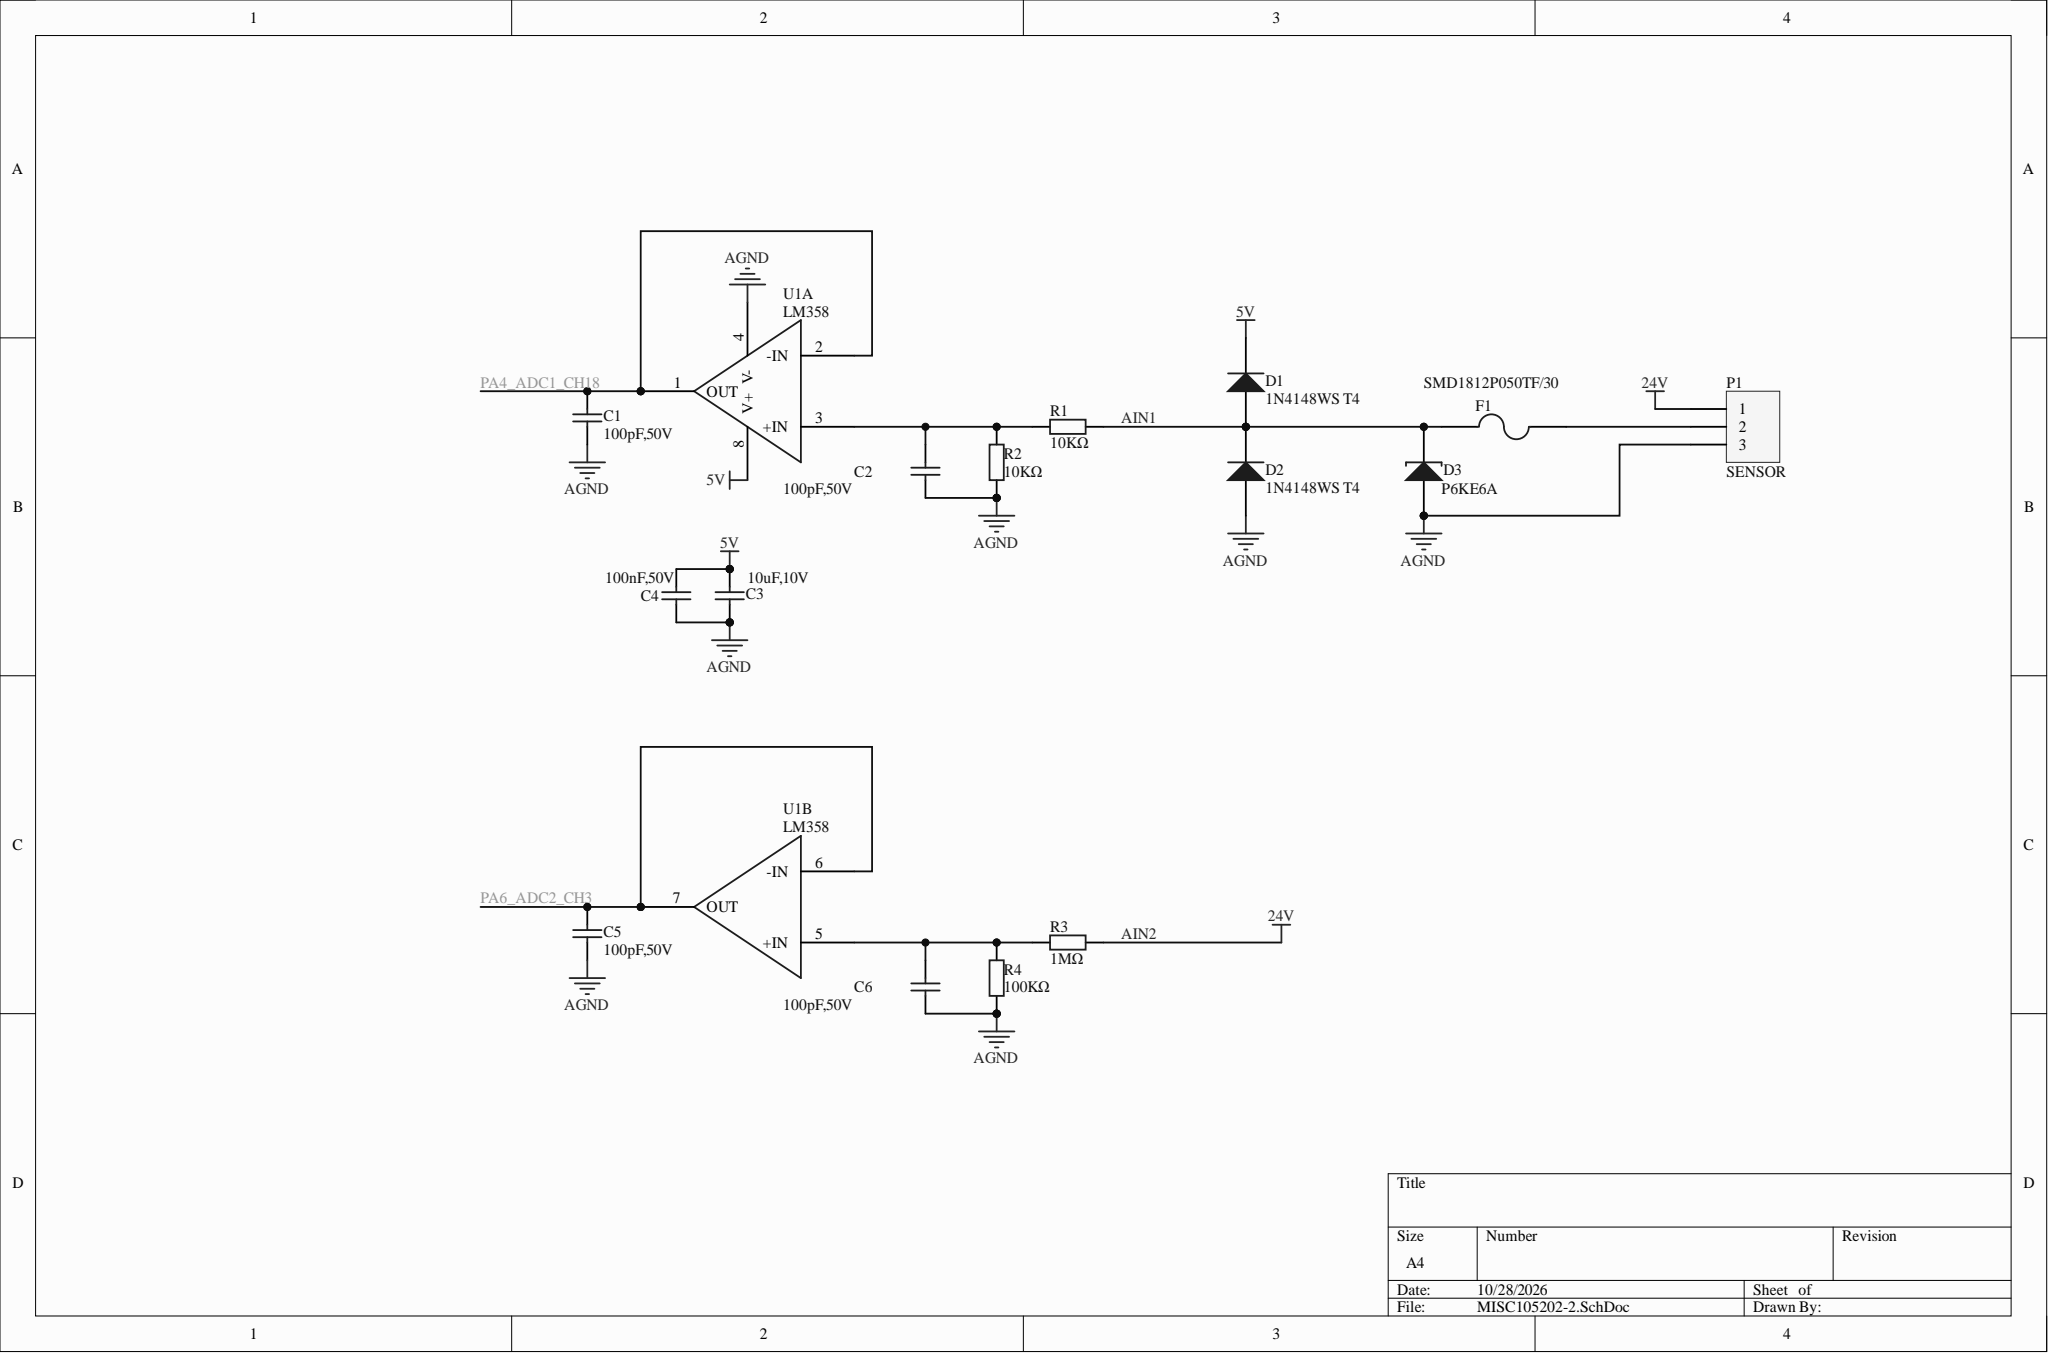Circuit board | Altium Designer | 181 parts | 141 nets | one sheet of the schematic
Parts on this sheet (reference | value | footprint):
C1 | 100pF,50V | 0603_C
C2 | 100pF,50V | 0603_C
C3 | 10uF,10V | 0603_C
C4 | 100nF,50V | 0603_C
C5 | 100pF,50V | 0603_C
C6 | 100pF,50V | 0603_C
D1 | 1N4148WS T4 | SOD-323
D2 | 1N4148WS T4 | SOD-323
D3 | P6KE6A | P6KESMD
F1 | SMD1812P050TF/30 | 1812
P1 | SENSOR | 508*3
R1 | 10KΩ | 0603_R
R2 | 10KΩ | 0603_R
R3 | 1MΩ | 0603_R
R4 | 100KΩ | 0603_R
Nets of these parts (net: part-pin ...):
PA6_ADC2_CH3: C5-2
PA4_ADC1_CH18: C1-2
NetF1_1: F1-1 P1-2
NetC6_2: C6-2 R3-1 R4-2
NetC2_2: C2-2 R1-1 R2-2
AIN2: P1-1 R3-2
AIN1: D1-1 D2-2 D3-2 F1-2 R1-2
AGND: C1-1 C2-1 C3-1 C4-1 C5-1 C6-1 D2-1 D3-1 P1-3 R2-1 R4-1
5V: C3-2 C4-2 D1-2